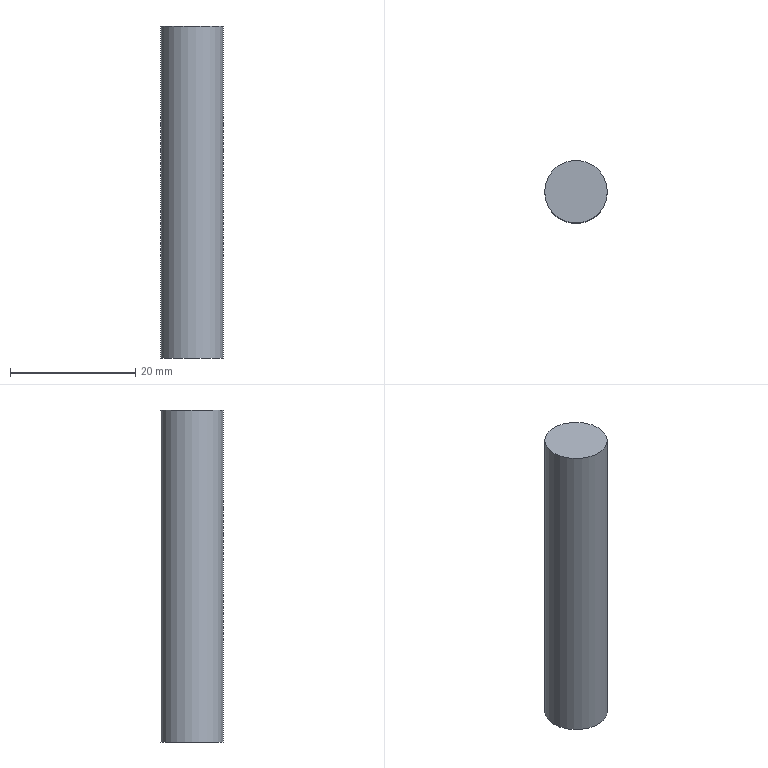Part | NX | features solid 2 | 1 solid | 3 faces | box 10 x 10 x 53 mm | volume 4163 mm3 | plane 2 | cylinder 1 | commonest cylinder face diameters 10 x1
STEP:
#1=CARTESIAN_POINT('',(-5.,-15.,85.5));
#2=VERTEX_POINT('',#1);
#3=CARTESIAN_POINT('',(0.,-15.,85.5));
#4=DIRECTION('',(0.,0.,-1.));
#5=DIRECTION('',(-1.,0.,0.));
#6=AXIS2_PLACEMENT_3D('',#3,#4,#5);
#7=CIRCLE('',#6,5.);
#8=EDGE_CURVE('',#2,#2,#7,.T.);
#9=ORIENTED_EDGE('',*,*,#8,.T.);
#10=EDGE_LOOP('',(#9));
#11=FACE_BOUND('',#10,.T.);
#12=CARTESIAN_POINT('',(-5.,-15.,32.5));
#13=VERTEX_POINT('',#12);
#14=CARTESIAN_POINT('',(0.,-15.,32.5));
#15=DIRECTION('',(0.,0.,-1.));
#16=DIRECTION('',(-1.,0.,0.));
#17=AXIS2_PLACEMENT_3D('',#14,#15,#16);
#18=CIRCLE('',#17,5.);
#19=EDGE_CURVE('',#13,#13,#18,.T.);
#20=ORIENTED_EDGE('',*,*,#19,.F.);
#21=EDGE_LOOP('',(#20));
#22=FACE_BOUND('',#21,.T.);
#23=CARTESIAN_POINT('',(0.,-15.,82.5));
#24=DIRECTION('',(0.,0.,-1.));
#25=DIRECTION('',(-1.,0.,0.));
#26=AXIS2_PLACEMENT_3D('',#23,#24,#25);
#27=CYLINDRICAL_SURFACE('',#26,5.);
#28=ADVANCED_FACE('',(#11,#22),#27,.T.);
#29=ORIENTED_EDGE('',*,*,#8,.F.);
#30=EDGE_LOOP('',(#29));
#31=FACE_BOUND('',#30,.T.);
#32=CARTESIAN_POINT('',(0.,-15.,85.5));
#33=DIRECTION('',(0.,0.,-1.));
#34=DIRECTION('',(-1.,0.,0.));
#35=AXIS2_PLACEMENT_3D('',#32,#33,#34);
#36=PLANE('',#35);
#37=ADVANCED_FACE('',(#31),#36,.F.);
#38=ORIENTED_EDGE('',*,*,#19,.T.);
#39=EDGE_LOOP('',(#38));
#40=FACE_BOUND('',#39,.T.);
#41=CARTESIAN_POINT('',(0.,-15.,32.5));
#42=DIRECTION('',(0.,0.,-1.));
#43=DIRECTION('',(-1.,0.,0.));
#44=AXIS2_PLACEMENT_3D('',#41,#42,#43);
#45=PLANE('',#44);
#46=ADVANCED_FACE('',(#40),#45,.T.);
#47=CLOSED_SHELL('',(#28,#37,#46));
#48=MANIFOLD_SOLID_BREP('',#47);
#49=(LENGTH_UNIT()NAMED_UNIT(*)SI_UNIT(.MILLI.,.METRE.));
#50=UNCERTAINTY_MEASURE_WITH_UNIT(LENGTH_MEASURE(0.00001),#49,'','');
#51=(NAMED_UNIT(*)PLANE_ANGLE_UNIT()SI_UNIT($,.RADIAN.));
#52=(NAMED_UNIT(*)SI_UNIT($,.STERADIAN.)SOLID_ANGLE_UNIT());
#53=(GEOMETRIC_REPRESENTATION_CONTEXT(3)GLOBAL_UNCERTAINTY_ASSIGNED_CONTEXT((#50))GLOBAL_UNIT_ASSIGNED_CONTEXT((#49,#51,#52))REPRESENTATION_CONTEXT('',''));
#54=ADVANCED_BREP_SHAPE_REPRESENTATION('',(#48),#53);